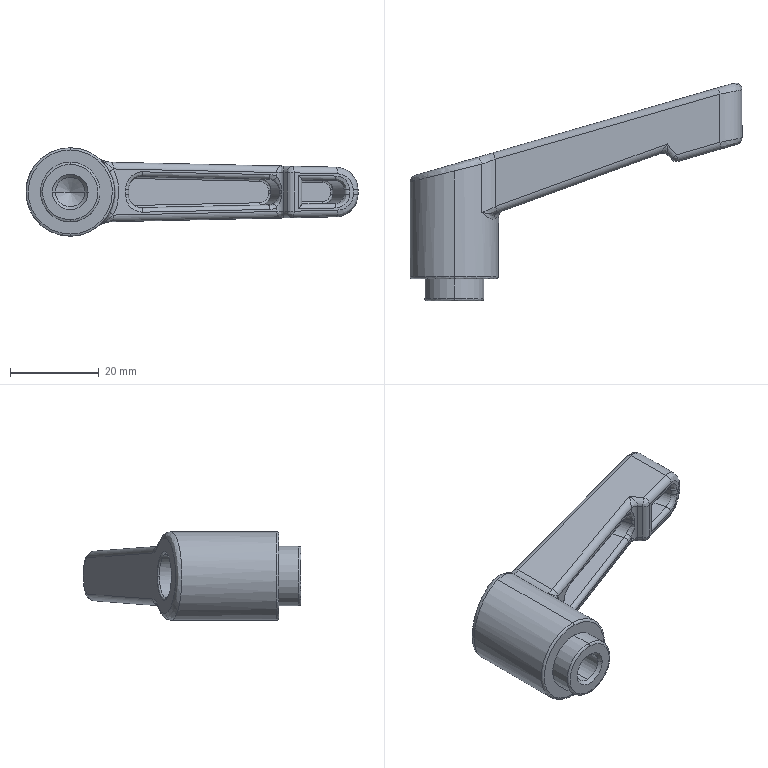Part | SolidWorks | features BaseBody 1 | 1 solid | 112 faces | box 75 x 49.204 x 20.002 mm | volume 13686 mm3 | cylinder 46 | spline 42 | plane 20 | cone 4 | commonest cylinder face diameters 3 x12 2 x10 1 x8 10 x4 5 x2 6 x2